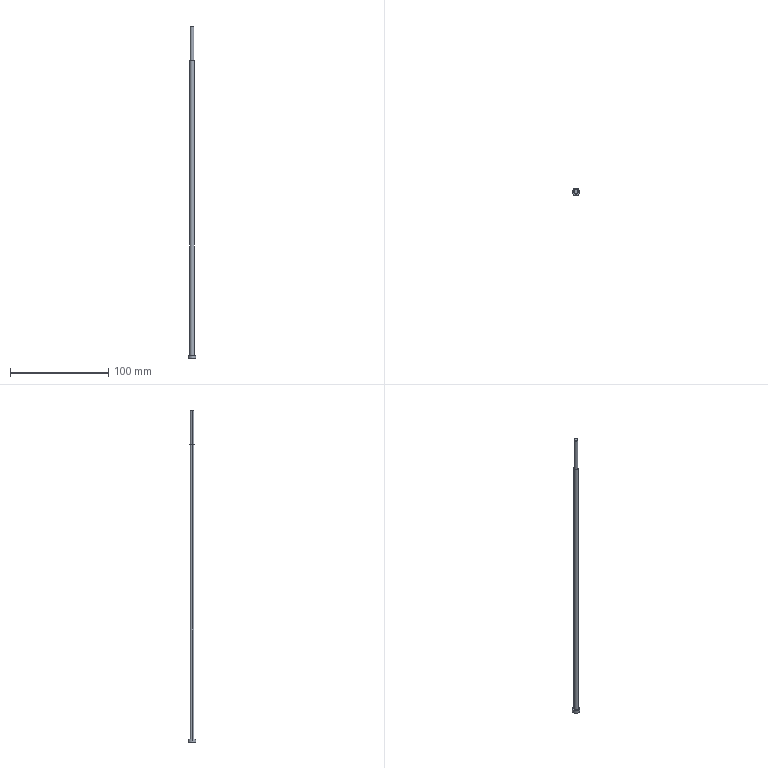Part | Creo | 1 solid | 11 faces | box 8 x 8 x 337.48 mm | volume 5352 mm3 | cylinder 6 | plane 3 | cone 2 | commonest cylinder face diameters 4 x2 4.5 x2 8 x2
STEP:
#1=CARTESIAN_POINT('',(-181.984,-198.792,7.486));
#2=VERTEX_POINT('',#1);
#3=CARTESIAN_POINT('',(-186.484,-198.792,7.486));
#4=VERTEX_POINT('',#3);
#5=CARTESIAN_POINT('',(-184.234,-198.792,7.486));
#6=DIRECTION('',(0.,0.,1.));
#7=DIRECTION('',(1.,0.,0.));
#8=AXIS2_PLACEMENT_3D('',#5,#6,#7);
#9=CIRCLE('',#8,2.25);
#10=EDGE_CURVE('',#2,#4,#9,.T.);
#11=ORIENTED_EDGE('',*,*,#10,.T.);
#12=CARTESIAN_POINT('',(-186.484,-198.792,-291.5));
#13=VERTEX_POINT('',#12);
#14=CARTESIAN_POINT('',(-186.484,-198.792,-291.5));
#15=DIRECTION('',(0.,0.,1.));
#16=VECTOR('',#15,298.986);
#17=LINE('',#14,#16);
#18=EDGE_CURVE('',#13,#4,#17,.T.);
#19=ORIENTED_EDGE('',*,*,#18,.F.);
#20=CARTESIAN_POINT('',(-181.984,-198.792,-291.5));
#21=VERTEX_POINT('',#20);
#22=CARTESIAN_POINT('',(-184.234,-198.792,-291.5));
#23=DIRECTION('',(0.,0.,-1.));
#24=DIRECTION('',(-1.,0.,0.));
#25=AXIS2_PLACEMENT_3D('',#22,#23,#24);
#26=CIRCLE('',#25,2.25);
#27=EDGE_CURVE('',#13,#21,#26,.T.);
#28=ORIENTED_EDGE('',*,*,#27,.T.);
#29=CARTESIAN_POINT('',(-181.984,-198.792,-291.5));
#30=DIRECTION('',(0.,0.,1.));
#31=VECTOR('',#30,298.986);
#32=LINE('',#29,#31);
#33=EDGE_CURVE('',#21,#2,#32,.T.);
#34=ORIENTED_EDGE('',*,*,#33,.T.);
#35=EDGE_LOOP('',(#11,#19,#28,#34));
#36=FACE_OUTER_BOUND('',#35,.F.);
#37=CARTESIAN_POINT('',(-184.234,-198.792,6.697));
#38=DIRECTION('',(0.,0.,1.));
#39=DIRECTION('',(1.,0.,0.));
#40=AXIS2_PLACEMENT_3D('',#37,#38,#39);
#41=CYLINDRICAL_SURFACE('',#40,2.25);
#42=ADVANCED_FACE('',(#36),#41,.T.);
#43=ORIENTED_EDGE('',*,*,#10,.F.);
#44=CARTESIAN_POINT('',(-182.234,-198.792,7.736));
#45=VERTEX_POINT('',#44);
#46=CARTESIAN_POINT('',(-182.234,-198.792,7.736));
#47=DIRECTION('',(0.7071,0.,-0.7071));
#48=VECTOR('',#47,0.3536);
#49=LINE('',#46,#48);
#50=EDGE_CURVE('',#45,#2,#49,.T.);
#51=ORIENTED_EDGE('',*,*,#50,.F.);
#52=CARTESIAN_POINT('',(-186.234,-198.792,7.736));
#53=VERTEX_POINT('',#52);
#54=CARTESIAN_POINT('',(-184.234,-198.792,7.736));
#55=DIRECTION('',(0.,0.,-1.));
#56=DIRECTION('',(-1.,0.,0.));
#57=AXIS2_PLACEMENT_3D('',#54,#55,#56);
#58=CIRCLE('',#57,2.);
#59=EDGE_CURVE('',#53,#45,#58,.T.);
#60=ORIENTED_EDGE('',*,*,#59,.F.);
#61=CARTESIAN_POINT('',(-186.234,-198.792,7.736));
#62=DIRECTION('',(-0.7071,0.,-0.7071));
#63=VECTOR('',#62,0.3536);
#64=LINE('',#61,#63);
#65=EDGE_CURVE('',#53,#4,#64,.T.);
#66=ORIENTED_EDGE('',*,*,#65,.T.);
#67=EDGE_LOOP('',(#43,#51,#60,#66));
#68=FACE_OUTER_BOUND('',#67,.F.);
#69=CARTESIAN_POINT('',(-184.234,-198.792,7.611));
#70=DIRECTION('',(0.,0.,-1.));
#71=DIRECTION('',(-1.,0.,0.));
#72=AXIS2_PLACEMENT_3D('',#69,#70,#71);
#73=CONICAL_SURFACE('',#72,2.125,45.);
#74=ADVANCED_FACE('',(#68),#73,.T.);
#75=CARTESIAN_POINT('',(-184.234,-198.792,7.486));
#76=DIRECTION('',(0.,0.,1.));
#77=DIRECTION('',(-1.,0.,0.));
#78=AXIS2_PLACEMENT_3D('',#75,#76,#77);
#79=CIRCLE('',#78,2.25);
#80=EDGE_CURVE('',#4,#2,#79,.T.);
#81=ORIENTED_EDGE('',*,*,#80,.F.);
#82=ORIENTED_EDGE('',*,*,#65,.F.);
#83=CARTESIAN_POINT('',(-184.234,-198.792,7.736));
#84=DIRECTION('',(0.,0.,-1.));
#85=DIRECTION('',(1.,0.,0.));
#86=AXIS2_PLACEMENT_3D('',#83,#84,#85);
#87=CIRCLE('',#86,2.);
#88=EDGE_CURVE('',#45,#53,#87,.T.);
#89=ORIENTED_EDGE('',*,*,#88,.F.);
#90=ORIENTED_EDGE('',*,*,#50,.T.);
#91=EDGE_LOOP('',(#81,#82,#89,#90));
#92=FACE_OUTER_BOUND('',#91,.F.);
#93=CARTESIAN_POINT('',(-184.234,-198.792,7.611));
#94=DIRECTION('',(0.,0.,-1.));
#95=DIRECTION('',(-1.,0.,0.));
#96=AXIS2_PLACEMENT_3D('',#93,#94,#95);
#97=CONICAL_SURFACE('',#96,2.125,45.);
#98=ADVANCED_FACE('',(#92),#97,.T.);
#99=ORIENTED_EDGE('',*,*,#80,.T.);
#100=ORIENTED_EDGE('',*,*,#33,.F.);
#101=CARTESIAN_POINT('',(-184.234,-198.792,-291.5));
#102=DIRECTION('',(0.,0.,-1.));
#103=DIRECTION('',(1.,0.,0.));
#104=AXIS2_PLACEMENT_3D('',#101,#102,#103);
#105=CIRCLE('',#104,2.25);
#106=EDGE_CURVE('',#21,#13,#105,.T.);
#107=ORIENTED_EDGE('',*,*,#106,.T.);
#108=ORIENTED_EDGE('',*,*,#18,.T.);
#109=EDGE_LOOP('',(#99,#100,#107,#108));
#110=FACE_OUTER_BOUND('',#109,.F.);
#111=CARTESIAN_POINT('',(-184.234,-198.792,6.697));
#112=DIRECTION('',(0.,0.,1.));
#113=DIRECTION('',(1.,0.,0.));
#114=AXIS2_PLACEMENT_3D('',#111,#112,#113);
#115=CYLINDRICAL_SURFACE('',#114,2.25);
#116=ADVANCED_FACE('',(#110),#115,.T.);
#117=CARTESIAN_POINT('',(-180.234,-198.792,-291.5));
#118=VERTEX_POINT('',#117);
#119=CARTESIAN_POINT('',(-188.234,-198.792,-291.5));
#120=VERTEX_POINT('',#119);
#121=CARTESIAN_POINT('',(-184.234,-198.792,-291.5));
#122=DIRECTION('',(0.,0.,1.));
#123=DIRECTION('',(1.,0.,0.));
#124=AXIS2_PLACEMENT_3D('',#121,#122,#123);
#125=CIRCLE('',#124,4.);
#126=EDGE_CURVE('',#118,#120,#125,.T.);
#127=ORIENTED_EDGE('',*,*,#126,.F.);
#128=CARTESIAN_POINT('',(-184.234,-198.792,-291.5));
#129=DIRECTION('',(0.,0.,1.));
#130=DIRECTION('',(-1.,0.,0.));
#131=AXIS2_PLACEMENT_3D('',#128,#129,#130);
#132=CIRCLE('',#131,4.);
#133=EDGE_CURVE('',#120,#118,#132,.T.);
#134=ORIENTED_EDGE('',*,*,#133,.F.);
#135=EDGE_LOOP('',(#127,#134));
#136=FACE_OUTER_BOUND('',#135,.F.);
#137=ORIENTED_EDGE('',*,*,#106,.F.);
#138=ORIENTED_EDGE('',*,*,#27,.F.);
#139=EDGE_LOOP('',(#137,#138));
#140=FACE_BOUND('',#139,.F.);
#141=CARTESIAN_POINT('',(-184.234,-198.792,-291.5));
#142=DIRECTION('',(0.,0.,1.));
#143=DIRECTION('',(-1.,0.,0.));
#144=AXIS2_PLACEMENT_3D('',#141,#142,#143);
#145=PLANE('',#144);
#146=ADVANCED_FACE('',(#136,#140),#145,.T.);
#147=ORIENTED_EDGE('',*,*,#126,.T.);
#148=CARTESIAN_POINT('',(-188.234,-198.792,-294.5));
#149=VERTEX_POINT('',#148);
#150=CARTESIAN_POINT('',(-188.234,-198.792,-294.5));
#151=DIRECTION('',(0.,0.,1.));
#152=VECTOR('',#151,3.);
#153=LINE('',#150,#152);
#154=EDGE_CURVE('',#149,#120,#153,.T.);
#155=ORIENTED_EDGE('',*,*,#154,.F.);
#156=CARTESIAN_POINT('',(-180.234,-198.792,-294.5));
#157=VERTEX_POINT('',#156);
#158=CARTESIAN_POINT('',(-184.234,-198.792,-294.5));
#159=DIRECTION('',(0.,0.,-1.));
#160=DIRECTION('',(-1.,0.,0.));
#161=AXIS2_PLACEMENT_3D('',#158,#159,#160);
#162=CIRCLE('',#161,4.);
#163=EDGE_CURVE('',#149,#157,#162,.T.);
#164=ORIENTED_EDGE('',*,*,#163,.T.);
#165=CARTESIAN_POINT('',(-180.234,-198.792,-294.5));
#166=DIRECTION('',(0.,0.,1.));
#167=VECTOR('',#166,3.);
#168=LINE('',#165,#167);
#169=EDGE_CURVE('',#157,#118,#168,.T.);
#170=ORIENTED_EDGE('',*,*,#169,.T.);
#171=EDGE_LOOP('',(#147,#155,#164,#170));
#172=FACE_OUTER_BOUND('',#171,.F.);
#173=CARTESIAN_POINT('',(-184.234,-198.792,-294.5));
#174=DIRECTION('',(0.,0.,1.));
#175=DIRECTION('',(-1.,0.,0.));
#176=AXIS2_PLACEMENT_3D('',#173,#174,#175);
#177=CYLINDRICAL_SURFACE('',#176,4.);
#178=ADVANCED_FACE('',(#172),#177,.T.);
#179=ORIENTED_EDGE('',*,*,#133,.T.);
#180=ORIENTED_EDGE('',*,*,#169,.F.);
#181=CARTESIAN_POINT('',(-184.234,-198.792,-294.5));
#182=DIRECTION('',(0.,0.,-1.));
#183=DIRECTION('',(1.,0.,0.));
#184=AXIS2_PLACEMENT_3D('',#181,#182,#183);
#185=CIRCLE('',#184,4.);
#186=EDGE_CURVE('',#157,#149,#185,.T.);
#187=ORIENTED_EDGE('',*,*,#186,.T.);
#188=ORIENTED_EDGE('',*,*,#154,.T.);
#189=EDGE_LOOP('',(#179,#180,#187,#188));
#190=FACE_OUTER_BOUND('',#189,.F.);
#191=CARTESIAN_POINT('',(-184.234,-198.792,-294.5));
#192=DIRECTION('',(0.,0.,1.));
#193=DIRECTION('',(-1.,0.,0.));
#194=AXIS2_PLACEMENT_3D('',#191,#192,#193);
#195=CYLINDRICAL_SURFACE('',#194,4.);
#196=ADVANCED_FACE('',(#190),#195,.T.);
#197=ORIENTED_EDGE('',*,*,#163,.F.);
#198=ORIENTED_EDGE('',*,*,#186,.F.);
#199=EDGE_LOOP('',(#197,#198));
#200=FACE_OUTER_BOUND('',#199,.F.);
#201=CARTESIAN_POINT('',(328.451,-835.47,-294.5));
#202=DIRECTION('',(0.,0.,-1.));
#203=DIRECTION('',(1.,0.,0.));
#204=AXIS2_PLACEMENT_3D('',#201,#202,#203);
#205=PLANE('',#204);
#206=ADVANCED_FACE('',(#200),#205,.T.);
#207=CARTESIAN_POINT('',(-186.234,-198.792,42.98));
#208=VERTEX_POINT('',#207);
#209=CARTESIAN_POINT('',(-182.234,-198.792,42.98));
#210=VERTEX_POINT('',#209);
#211=CARTESIAN_POINT('',(-184.234,-198.792,42.98));
#212=DIRECTION('',(0.,0.,1.));
#213=DIRECTION('',(-1.,0.,0.));
#214=AXIS2_PLACEMENT_3D('',#211,#212,#213);
#215=CIRCLE('',#214,2.);
#216=EDGE_CURVE('',#208,#210,#215,.T.);
#217=ORIENTED_EDGE('',*,*,#216,.T.);
#218=CARTESIAN_POINT('',(-182.234,-198.792,7.736));
#219=DIRECTION('',(0.,0.,1.));
#220=VECTOR('',#219,35.244);
#221=LINE('',#218,#220);
#222=EDGE_CURVE('',#45,#210,#221,.T.);
#223=ORIENTED_EDGE('',*,*,#222,.F.);
#224=ORIENTED_EDGE('',*,*,#88,.T.);
#225=CARTESIAN_POINT('',(-186.234,-198.792,7.736));
#226=DIRECTION('',(0.,0.,1.));
#227=VECTOR('',#226,35.244);
#228=LINE('',#225,#227);
#229=EDGE_CURVE('',#53,#208,#228,.T.);
#230=ORIENTED_EDGE('',*,*,#229,.T.);
#231=EDGE_LOOP('',(#217,#223,#224,#230));
#232=FACE_OUTER_BOUND('',#231,.F.);
#233=CARTESIAN_POINT('',(-184.234,-198.792,6.697));
#234=DIRECTION('',(0.,0.,1.));
#235=DIRECTION('',(1.,0.,0.));
#236=AXIS2_PLACEMENT_3D('',#233,#234,#235);
#237=CYLINDRICAL_SURFACE('',#236,2.);
#238=ADVANCED_FACE('',(#232),#237,.T.);
#239=CARTESIAN_POINT('',(-184.234,-198.792,42.98));
#240=DIRECTION('',(0.,0.,1.));
#241=DIRECTION('',(1.,0.,0.));
#242=AXIS2_PLACEMENT_3D('',#239,#240,#241);
#243=CIRCLE('',#242,2.);
#244=EDGE_CURVE('',#210,#208,#243,.T.);
#245=ORIENTED_EDGE('',*,*,#244,.F.);
#246=ORIENTED_EDGE('',*,*,#216,.F.);
#247=EDGE_LOOP('',(#245,#246));
#248=FACE_OUTER_BOUND('',#247,.F.);
#249=CARTESIAN_POINT('',(-46.549,-435.469,42.98));
#250=DIRECTION('',(0.,0.,1.));
#251=DIRECTION('',(0.,-1.,0.));
#252=AXIS2_PLACEMENT_3D('',#249,#250,#251);
#253=PLANE('',#252);
#254=ADVANCED_FACE('',(#248),#253,.T.);
#255=ORIENTED_EDGE('',*,*,#244,.T.);
#256=ORIENTED_EDGE('',*,*,#229,.F.);
#257=ORIENTED_EDGE('',*,*,#59,.T.);
#258=ORIENTED_EDGE('',*,*,#222,.T.);
#259=EDGE_LOOP('',(#255,#256,#257,#258));
#260=FACE_OUTER_BOUND('',#259,.F.);
#261=CARTESIAN_POINT('',(-184.234,-198.792,6.697));
#262=DIRECTION('',(0.,0.,1.));
#263=DIRECTION('',(1.,0.,0.));
#264=AXIS2_PLACEMENT_3D('',#261,#262,#263);
#265=CYLINDRICAL_SURFACE('',#264,2.);
#266=ADVANCED_FACE('',(#260),#265,.T.);
#267=CLOSED_SHELL('',(#42,#74,#98,#116,#146,#178,#196,#206,#238,#254,#266));
#268=MANIFOLD_SOLID_BREP('',#267);
#269=(LENGTH_UNIT()NAMED_UNIT(*)SI_UNIT(.MILLI.,.METRE.));
#270=UNCERTAINTY_MEASURE_WITH_UNIT(LENGTH_MEASURE(0.03377),#269,'','');
#271=(NAMED_UNIT(*)PLANE_ANGLE_UNIT()SI_UNIT($,.RADIAN.));
#272=PLANE_ANGLE_MEASURE_WITH_UNIT(PLANE_ANGLE_MEASURE(0.01745),#271);
#273=(CONVERSION_BASED_UNIT('DEGREE',#272)NAMED_UNIT(*)PLANE_ANGLE_UNIT());
#274=(NAMED_UNIT(*)SI_UNIT($,.STERADIAN.)SOLID_ANGLE_UNIT());
#275=(GEOMETRIC_REPRESENTATION_CONTEXT(3)GLOBAL_UNCERTAINTY_ASSIGNED_CONTEXT((#270))GLOBAL_UNIT_ASSIGNED_CONTEXT((#269,#273,#274))REPRESENTATION_CONTEXT('',''));
#276=ADVANCED_BREP_SHAPE_REPRESENTATION('',(#268),#275);